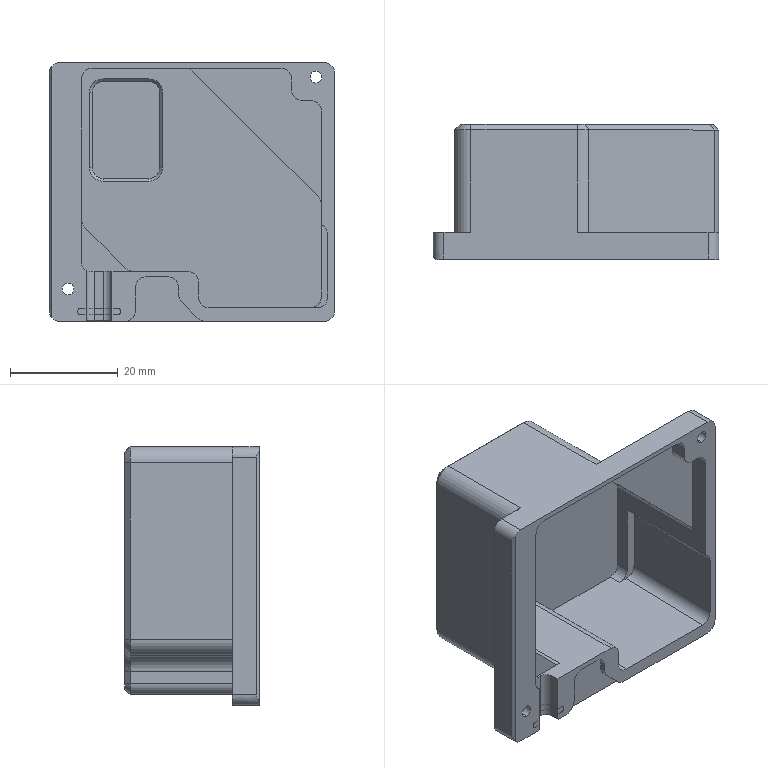NC program | NX | posted with a generic post | part box 53 x 25 x 48 mm
Lines 1678 to 3424 of 6007:
(PLANAR_MILL_3 , TOOL : D4-12-D4-50-3T-ROUGH)
N3348 T09 M6
N3350 G54
N3352 G17 G0 G90 X-17.741 Y0.375 B0. C0. S3000 M3
N3354 G43 Z30. H9
N3356 Z1.004 B-180. C-180.
N3358 G94 G1 Z-0.996 F600.
N3360 X-19.005 Y0.525
N3362 X-19.033 Y0.497
N3364 X-20.9 Y-1.37
N3366 Y-4.009
N3368 Y-4.049
N3370 X-19.9 Y-4.838
N3372 Z1.004
N3374 G0 X-17.741 Y0.375 Z0.009
N3376 G1 Z-1.991
N3378 X-19.005 Y0.525
N3380 X-19.033 Y0.497
N3382 X-20.9 Y-1.37
N3384 Y-4.009
N3386 Y-4.049
N3388 X-19.9 Y-4.838
N3390 Z0.009
N3392 G0 X-17.741 Y0.375 Z-0.987
N3394 G1 Z-2.987
N3396 X-19.005 Y0.525
N3398 X-19.033 Y0.497
N3400 X-20.9 Y-1.37
N3402 Y-4.009
N3404 Y-4.049
N3406 X-19.9 Y-4.838
N3408 Z-0.987
N3410 G0 X-17.741 Y0.375 Z-1.983
N3412 G1 Z-3.983
N3414 X-19.005 Y0.525
N3416 X-19.033 Y0.497
N3418 X-20.9 Y-1.37
N3420 Y-4.009
N3422 Y-4.049
N3424 X-19.9 Y-4.838
N3426 Z-1.983
N3428 G0 X-17.741 Y0.375 Z-2.978
N3430 G1 Z-4.978
N3432 X-19.005 Y0.525
N3434 X-19.033 Y0.497
N3436 X-20.9 Y-1.37
N3438 Y-4.009
N3440 Y-4.049
N3442 X-19.9 Y-4.838
N3444 Z-2.978
N3446 G0 X-17.741 Y0.375 Z-3.974
N3448 G1 Z-5.974
N3450 X-19.005 Y0.525
N3452 X-19.033 Y0.497
N3454 X-20.9 Y-1.37
N3456 Y-4.009
N3458 Y-4.049
N3460 X-19.9 Y-4.838
N3462 Z-3.974
N3464 G0 X-17.741 Y0.375 Z-4.97
N3466 G1 Z-6.97
N3468 X-19.005 Y0.525
N3470 X-19.033 Y0.497
N3472 X-20.9 Y-1.37
N3474 Y-4.009
N3476 Y-4.049
N3478 X-19.9 Y-4.838
N3480 Z-4.97
N3482 G0 X-17.741 Y0.375 Z-5.965
N3484 G1 Z-7.965
N3486 X-19.005 Y0.525
N3488 X-19.033 Y0.497
N3490 X-20.9 Y-1.37
N3492 Y-4.009
N3494 Y-4.049
N3496 X-19.9 Y-4.838
N3498 Z-5.965
N3500 G0 X-17.741 Y0.375 Z-6.961
N3502 G1 Z-8.961
N3504 X-19.005 Y0.525
N3506 X-19.033 Y0.497
N3508 X-20.9 Y-1.37
N3510 Y-4.009
N3512 Y-4.049
N3514 X-19.9 Y-4.838
N3516 Z-6.961
N3518 G0 X-17.741 Y0.375 Z-7.957
N3520 G1 Z-9.957
N3522 X-19.005 Y0.525
N3524 X-19.033 Y0.497
N3526 X-20.9 Y-1.37
N3528 Y-4.009
N3530 Y-4.049
N3532 X-19.9 Y-4.838
N3534 Z-7.957
N3536 G0 X-17.741 Y0.375 Z-8.952
N3538 G1 Z-10.952
N3540 X-19.005 Y0.525
N3542 X-19.033 Y0.497
N3544 X-20.9 Y-1.37
N3546 Y-4.009
N3548 Y-4.049
N3550 X-19.9 Y-4.838
N3552 Z-8.952
N3554 G0 X-17.741 Y0.375 Z-9.948
N3556 G1 Z-11.948
N3558 X-19.005 Y0.525
N3560 X-19.033 Y0.497
N3562 X-20.9 Y-1.37
N3564 Y-4.009
N3566 Y-4.049
N3568 X-19.9 Y-4.838
N3570 Z-9.948
N3572 G0 X-17.741 Y0.375 Z-10.943
N3574 G1 Z-12.943
N3576 X-19.005 Y0.525
N3578 X-19.033 Y0.497
N3580 X-20.9 Y-1.37
N3582 Y-4.009
N3584 Y-4.049
N3586 X-19.9 Y-4.838
N3588 Z-10.943
N3590 G0 X-17.741 Y0.375 Z-11.939
N3592 G1 Z-13.939
N3594 X-19.005 Y0.525
N3596 X-19.033 Y0.497
N3598 X-20.9 Y-1.37
N3600 Y-4.009
N3602 Y-4.049
N3604 X-19.9 Y-4.838
N3606 Z-11.939
N3608 G0 X-17.741 Y0.375 Z-12.935
N3610 G1 Z-14.935
N3612 X-19.005 Y0.525
N3614 X-19.033 Y0.497
N3616 X-20.9 Y-1.37
N3618 Y-4.009
N3620 Y-4.049
N3622 X-19.9 Y-4.838
N3624 Z-12.935
N3626 G0 X-17.741 Y0.375 Z-13.93
N3628 G1 Z-15.93
N3630 X-19.005 Y0.525
N3632 X-19.033 Y0.497
N3634 X-20.9 Y-1.37
N3636 Y-4.009
N3638 Y-4.049
N3640 X-19.9 Y-4.838
N3642 Z-13.93
N3644 G0 X-17.741 Y0.375 Z-14.926
N3646 G1 Z-16.926
N3648 X-19.005 Y0.525
N3650 X-19.033 Y0.497
N3652 X-20.9 Y-1.37
N3654 Y-4.009
N3656 Y-4.049
N3658 X-19.9 Y-4.838
N3660 Z-14.926
N3662 G0 X-17.741 Y0.375 Z-15.922
N3664 G1 Z-17.922
N3666 X-19.005 Y0.525
N3668 X-19.033 Y0.497
N3670 X-20.9 Y-1.37
N3672 Y-4.009
N3674 Y-4.049
N3676 X-19.9 Y-4.838
N3678 Z-15.922
N3680 G0 X-17.741 Y0.375 Z-16.917
N3682 G1 Z-18.917
N3684 X-19.005 Y0.525
N3686 X-19.033 Y0.497
N3688 X-20.9 Y-1.37
N3690 Y-4.009
N3692 Y-4.049
N3694 X-19.9 Y-4.838
N3696 Z-16.917
N3698 G0 X-17.741 Y0.375 Z-17.913
N3700 G1 Z-19.913
N3702 X-19.005 Y0.525
N3704 X-19.033 Y0.497
N3706 X-20.9 Y-1.37
N3708 Y-4.009
N3710 Y-4.049
N3712 X-19.9 Y-4.838
N3714 Z-17.913
N3716 G0 X-17.741 Y0.375 Z-18.909
N3718 G1 Z-20.909
N3720 X-19.005 Y0.525
N3722 X-19.033 Y0.497
N3724 X-20.9 Y-1.37
N3726 Y-4.009
N3728 Y-4.049
N3730 X-19.9 Y-4.838
N3732 Z-18.909
N3734 G0 X-17.741 Y0.375 Z-19.904
N3736 G1 Z-21.904
N3738 X-19.005 Y0.525
N3740 X-19.033 Y0.497
N3742 X-20.9 Y-1.37
N3744 Y-4.009
N3746 Y-4.049
N3748 X-19.9 Y-4.838
N3750 Z-19.904
N3752 G0 X-17.741 Y0.375 Z-20.9
N3754 G1 Z-22.9
N3756 X-19.005 Y0.525
N3758 X-19.033 Y0.497
N3760 X-20.9 Y-1.37
N3762 Y-4.009
N3764 Y-4.049
N3766 X-19.9 Y-4.838
N3768 Z-20.9
N3770 G0 Z3.
N3772 Y-13.175
N3774 Z1.004
N3776 G1 Z-0.996
N3778 X-20.9 Y-13.963
N3780 Y-14.003
N3782 Y-18.4
N3784 X-16.503
N3786 X-16.463
N3788 X-15.675 Y-17.4
N3790 Z1.004
N3792 G0 X-19.9 Y-13.175 Z0.009
N3794 G1 Z-1.991
N3796 X-20.9 Y-13.963
N3798 Y-14.003
N3800 Y-18.4
N3802 X-16.503
N3804 X-16.463
N3806 X-15.675 Y-17.4
N3808 Z0.009
N3810 G0 X-19.9 Y-13.175 Z-0.987
N3812 G1 Z-2.987
N3814 X-20.9 Y-13.963
N3816 Y-14.003
N3818 Y-18.4
N3820 X-16.503
N3822 X-16.463
N3824 X-15.675 Y-17.4
N3826 Z-0.987
N3828 G0 X-19.9 Y-13.175 Z-1.983
N3830 G1 Z-3.983
N3832 X-20.9 Y-13.963
N3834 Y-14.003
N3836 Y-18.4
N3838 X-16.503
N3840 X-16.463
N3842 X-15.675 Y-17.4
N3844 Z-1.983
N3846 G0 X-19.9 Y-13.175 Z-2.978
N3848 G1 Z-4.978
N3850 X-20.9 Y-13.963
N3852 Y-14.003
N3854 Y-18.4
N3856 X-16.503
N3858 X-16.463
N3860 X-15.675 Y-17.4
N3862 Z-2.978
N3864 G0 X-19.9 Y-13.175 Z-3.974
N3866 G1 Z-5.974
N3868 X-20.9 Y-13.963
N3870 Y-14.003
N3872 Y-18.4
N3874 X-16.503
N3876 X-16.463
N3878 X-15.675 Y-17.4
N3880 Z-3.974
N3882 G0 X-19.9 Y-13.175 Z-4.97
N3884 G1 Z-6.97
N3886 X-20.9 Y-13.963
N3888 Y-14.003
N3890 Y-18.4
N3892 X-16.503
N3894 X-16.463
N3896 X-15.675 Y-17.4
N3898 Z-4.97
N3900 G0 X-19.9 Y-13.175 Z-5.965
N3902 G1 Z-7.965
N3904 X-20.9 Y-13.963
N3906 Y-14.003
N3908 Y-18.4
N3910 X-16.503
N3912 X-16.463
N3914 X-15.675 Y-17.4
N3916 Z-5.965
N3918 G0 X-19.9 Y-13.175 Z-6.961
N3920 G1 Z-8.961
N3922 X-20.9 Y-13.963
N3924 Y-14.003
N3926 Y-18.4
N3928 X-16.503
N3930 X-16.463
N3932 X-15.675 Y-17.4
N3934 Z-6.961
N3936 G0 X-19.9 Y-13.175 Z-7.957
N3938 G1 Z-9.957
N3940 X-20.9 Y-13.963
N3942 Y-14.003
N3944 Y-18.4
N3946 X-16.503
N3948 X-16.463
N3950 X-15.675 Y-17.4
N3952 Z-7.957
N3954 G0 X-19.9 Y-13.175 Z-8.952
N3956 G1 Z-10.952
N3958 X-20.9 Y-13.963
N3960 Y-14.003
N3962 Y-18.4
N3964 X-16.503
N3966 X-16.463
N3968 X-15.675 Y-17.4
N3970 Z-8.952
N3972 G0 X-19.9 Y-13.175 Z-9.948
N3974 G1 Z-11.948
N3976 X-20.9 Y-13.963
N3978 Y-14.003
N3980 Y-18.4
N3982 X-16.503
N3984 X-16.463
N3986 X-15.675 Y-17.4
N3988 Z-9.948
N3990 G0 X-19.9 Y-13.175 Z-10.943
N3992 G1 Z-12.943
N3994 X-20.9 Y-13.963
N3996 Y-14.003
N3998 Y-18.4
N4000 X-16.503
N4002 X-16.463
N4004 X-15.675 Y-17.4
N4006 Z-10.943
N4008 G0 X-19.9 Y-13.175 Z-11.939
N4010 G1 Z-13.939
N4012 X-20.9 Y-13.963
N4014 Y-14.003
N4016 Y-18.4
N4018 X-16.503
N4020 X-16.463
N4022 X-15.675 Y-17.4
N4024 Z-11.939
N4026 G0 X-19.9 Y-13.175 Z-12.935
N4028 G1 Z-14.935
N4030 X-20.9 Y-13.963
N4032 Y-14.003
N4034 Y-18.4
N4036 X-16.503
N4038 X-16.463
N4040 X-15.675 Y-17.4
N4042 Z-12.935
N4044 G0 X-19.9 Y-13.175 Z-13.93
N4046 G1 Z-15.93
N4048 X-20.9 Y-13.963
N4050 Y-14.003
N4052 Y-18.4
N4054 X-16.503
N4056 X-16.463
N4058 X-15.675 Y-17.4
N4060 Z-13.93
N4062 G0 X-19.9 Y-13.175 Z-14.926
N4064 G1 Z-16.926
N4066 X-20.9 Y-13.963
N4068 Y-14.003
N4070 Y-18.4
N4072 X-16.503
N4074 X-16.463
N4076 X-15.675 Y-17.4
N4078 Z-14.926
N4080 G0 X-19.9 Y-13.175 Z-15.922
N4082 G1 Z-17.922
N4084 X-20.9 Y-13.963
N4086 Y-14.003
N4088 Y-18.4
N4090 X-16.503
N4092 X-16.463
N4094 X-15.675 Y-17.4
N4096 Z-15.922
N4098 G0 X-19.9 Y-13.175 Z-16.917
N4100 G1 Z-18.917
N4102 X-20.9 Y-13.963
N4104 Y-14.003
N4106 Y-18.4
N4108 X-16.503
N4110 X-16.463
N4112 X-15.675 Y-17.4
N4114 Z-16.917
N4116 G0 X-19.9 Y-13.175 Z-17.913
N4118 G1 Z-19.913
N4120 X-20.9 Y-13.963
N4122 Y-14.003
N4124 Y-18.4
N4126 X-16.503
N4128 X-16.463
N4130 X-15.675 Y-17.4
N4132 Z-17.913
N4134 G0 X-19.9 Y-13.175 Z-18.909
N4136 G1 Z-20.909
N4138 X-20.9 Y-13.963
N4140 Y-14.003
N4142 Y-18.4
N4144 X-16.503
N4146 X-16.463
N4148 X-15.675 Y-17.4
N4150 Z-18.909
N4152 G0 X-19.9 Y-13.175 Z-19.904
N4154 G1 Z-21.904
N4156 X-20.9 Y-13.963
N4158 Y-14.003
N4160 Y-18.4
N4162 X-16.503
N4164 X-16.463
N4166 X-15.675 Y-17.4
N4168 Z-19.904
N4170 G0 X-19.9 Y-13.175 Z-20.9
N4172 G1 Z-22.9
N4174 X-20.9 Y-13.963
N4176 Y-14.003
N4178 Y-18.4
N4180 X-16.503
N4182 X-16.463
N4184 X-15.675 Y-17.4
N4186 Z-20.9
N4188 G0 Z3.
N4190 X1.662
N4192 Z1.004
N4194 G1 Z-0.996
N4196 X2.451 Y-18.4
N4198 X2.491
N4200 X5.13
N4202 X6.997 Y-16.533
N4204 X7.025 Y-16.505
N4206 X6.875 Y-15.241
N4208 Z1.004
N4210 G0 X1.662 Y-17.4 Z0.009
N4212 G1 Z-1.991
N4214 X2.451 Y-18.4
N4216 X2.491
N4218 X5.13
N4220 X6.997 Y-16.533
N4222 X7.025 Y-16.505
N4224 X6.875 Y-15.241
N4226 Z0.009
N4228 G0 X1.662 Y-17.4 Z-0.987
N4230 G1 Z-2.987
N4232 X2.451 Y-18.4
N4234 X2.491
N4236 X5.13
N4238 X6.997 Y-16.533
N4240 X7.025 Y-16.505
N4242 X6.875 Y-15.241
N4244 Z-0.987
N4246 G0 X1.662 Y-17.4 Z-1.983
N4248 G1 Z-3.983
N4250 X2.451 Y-18.4
N4252 X2.491
N4254 X5.13
N4256 X6.997 Y-16.533
N4258 X7.025 Y-16.505
N4260 X6.875 Y-15.241
N4262 Z-1.983
N4264 G0 X1.662 Y-17.4 Z-2.978
N4266 G1 Z-4.978
N4268 X2.451 Y-18.4
N4270 X2.491
N4272 X5.13
N4274 X6.997 Y-16.533
N4276 X7.025 Y-16.505
N4278 X6.875 Y-15.241
N4280 Z-2.978
N4282 G0 X1.662 Y-17.4 Z-3.974
N4284 G1 Z-5.974
N4286 X2.451 Y-18.4
N4288 X2.491
N4290 X5.13
N4292 X6.997 Y-16.533
N4294 X7.025 Y-16.505
N4296 X6.875 Y-15.241
N4298 Z-3.974
N4300 G0 X1.662 Y-17.4 Z-4.97
N4302 G1 Z-6.97
N4304 X2.451 Y-18.4
N4306 X2.491
N4308 X5.13
N4310 X6.997 Y-16.533
N4312 X7.025 Y-16.505
N4314 X6.875 Y-15.241
N4316 Z-4.97
N4318 G0 X1.662 Y-17.4 Z-5.965
N4320 G1 Z-7.965
N4322 X2.451 Y-18.4
N4324 X2.491
N4326 X5.13
N4328 X6.997 Y-16.533
N4330 X7.025 Y-16.505
N4332 X6.875 Y-15.241
N4334 Z-5.965
N4336 G0 X1.662 Y-17.4 Z-6.961
N4338 G1 Z-8.961
N4340 X2.451 Y-18.4
N4342 X2.491
N4344 X5.13
N4346 X6.997 Y-16.533
N4348 X7.025 Y-16.505
N4350 X6.875 Y-15.241
N4352 Z-6.961
N4354 G0 X1.662 Y-17.4 Z-7.957
N4356 G1 Z-9.957
N4358 X2.451 Y-18.4
N4360 X2.491
N4362 X5.13
N4364 X6.997 Y-16.533
N4366 X7.025 Y-16.505
N4368 X6.875 Y-15.241
N4370 Z-7.957
N4372 G0 X1.662 Y-17.4 Z-8.952
N4374 G1 Z-10.952
N4376 X2.451 Y-18.4
N4378 X2.491
N4380 X5.13
N4382 X6.997 Y-16.533
N4384 X7.025 Y-16.505
N4386 X6.875 Y-15.241
N4388 Z-8.952
N4390 G0 X1.662 Y-17.4 Z-9.948
N4392 G1 Z-11.948
N4394 X2.451 Y-18.4
N4396 X2.491
N4398 X5.13
N4400 X6.997 Y-16.533
N4402 X7.025 Y-16.505
N4404 X6.875 Y-15.241
N4406 Z-9.948
N4408 G0 X1.662 Y-17.4 Z-10.943
N4410 G1 Z-12.943
N4412 X2.451 Y-18.4
N4414 X2.491
N4416 X5.13
N4418 X6.997 Y-16.533
N4420 X7.025 Y-16.505
N4422 X6.875 Y-15.241
N4424 Z-10.943
N4426 G0 X1.662 Y-17.4 Z-11.939
N4428 G1 Z-13.939
N4430 X2.451 Y-18.4
N4432 X2.491
N4434 X5.13
N4436 X6.997 Y-16.533
N4438 X7.025 Y-16.505
N4440 X6.875 Y-15.241
N4442 Z-11.939
N4444 G0 X1.662 Y-17.4 Z-12.935
N4446 G1 Z-14.935
N4448 X2.451 Y-18.4
N4450 X2.491
N4452 X5.13
N4454 X6.997 Y-16.533
N4456 X7.025 Y-16.505
N4458 X6.875 Y-15.241
N4460 Z-12.935
N4462 G0 X1.662 Y-17.4 Z-13.93
N4464 G1 Z-15.93
N4466 X2.451 Y-18.4
N4468 X2.491
N4470 X5.13
N4472 X6.997 Y-16.533
N4474 X7.025 Y-16.505
N4476 X6.875 Y-15.241
N4478 Z-13.93
N4480 G0 X1.662 Y-17.4 Z-14.926
N4482 G1 Z-16.926
N4484 X2.451 Y-18.4
N4486 X2.491
N4488 X5.13
N4490 X6.997 Y-16.533
N4492 X7.025 Y-16.505
N4494 X6.875 Y-15.241
N4496 Z-14.926
N4498 G0 X1.662 Y-17.4 Z-15.922
N4500 G1 Z-17.922
N4502 X2.451 Y-18.4
N4504 X2.491
N4506 X5.13
N4508 X6.997 Y-16.533
N4510 X7.025 Y-16.505
N4512 X6.875 Y-15.241
N4514 Z-15.922
N4516 G0 X1.662 Y-17.4 Z-16.917
N4518 G1 Z-18.917
N4520 X2.451 Y-18.4
N4522 X2.491
N4524 X5.13
N4526 X6.997 Y-16.533
N4528 X7.025 Y-16.505
N4530 X6.875 Y-15.241
N4532 Z-16.917
N4534 G0 X1.662 Y-17.4 Z-17.913
N4536 G1 Z-19.913
N4538 X2.451 Y-18.4
N4540 X2.491
N4542 X5.13
N4544 X6.997 Y-16.533
N4546 X7.025 Y-16.505
N4548 X6.875 Y-15.241
N4550 Z-17.913
N4552 G0 X1.662 Y-17.4 Z-18.909
N4554 G1 Z-20.909
N4556 X2.451 Y-18.4
N4558 X2.491
N4560 X5.13
N4562 X6.997 Y-16.533
N4564 X7.025 Y-16.505
N4566 X6.875 Y-15.241
N4568 Z-18.909
N4570 G0 X1.662 Y-17.4 Z-19.904
N4572 G1 Z-21.904
N4574 X2.451 Y-18.4
N4576 X2.491
N4578 X5.13
N4580 X6.997 Y-16.533
N4582 X7.025 Y-16.505
N4584 X6.875 Y-15.241
N4586 Z-19.904
N4588 G0 X1.662 Y-17.4 Z-20.9
N4590 G1 Z-22.9
N4592 X2.451 Y-18.4
N4594 X2.491
N4596 X5.13
N4598 X6.997 Y-16.533
N4600 X7.025 Y-16.505
N4602 X6.875 Y-15.241
N4604 Z-20.9
N4606 G0 Z3.
N4608 X9.491 Y-12.625
N4610 Z1.004
N4612 G1 Z-0.996
N4614 X10.755 Y-12.775
N4616 X10.783 Y-12.747
N4618 X12.65 Y-10.88
N4620 Y-8.241
N4622 Y-8.201
N4624 X11.65 Y-7.412
N4626 Z1.004
N4628 G0 X9.491 Y-12.625 Z0.009
N4630 G1 Z-1.991
N4632 X10.755 Y-12.775
N4634 X10.783 Y-12.747
N4636 X12.65 Y-10.88
N4638 Y-8.241
N4640 Y-8.201
N4642 X11.65 Y-7.412
N4644 Z0.009
N4646 G0 X9.491 Y-12.625 Z-0.987
N4648 G1 Z-2.987
N4650 X10.755 Y-12.775
N4652 X10.783 Y-12.747
N4654 X12.65 Y-10.88
N4656 Y-8.241
N4658 Y-8.201
N4660 X11.65 Y-7.412
N4662 Z-0.987
N4664 G0 X9.491 Y-12.625 Z-1.983
N4666 G1 Z-3.983
N4668 X10.755 Y-12.775
N4670 X10.783 Y-12.747
N4672 X12.65 Y-10.88
N4674 Y-8.241
N4676 Y-8.201
N4678 X11.65 Y-7.412
N4680 Z-1.983
N4682 G0 X9.491 Y-12.625 Z-2.978
N4684 G1 Z-4.978
N4686 X10.755 Y-12.775
N4688 X10.783 Y-12.747
N4690 X12.65 Y-10.88
N4692 Y-8.241
N4694 Y-8.201
N4696 X11.65 Y-7.412
N4698 Z-2.978
N4700 G0 X9.491 Y-12.625 Z-3.974
N4702 G1 Z-5.974
N4704 X10.755 Y-12.775
N4706 X10.783 Y-12.747
N4708 X12.65 Y-10.88
N4710 Y-8.241
N4712 Y-8.201
N4714 X11.65 Y-7.412
N4716 Z-3.974
N4718 G0 X9.491 Y-12.625 Z-4.97
N4720 G1 Z-6.97
N4722 X10.755 Y-12.775
N4724 X10.783 Y-12.747
N4726 X12.65 Y-10.88
N4728 Y-8.241
N4730 Y-8.201
N4732 X11.65 Y-7.412
N4734 Z-4.97
N4736 G0 X9.491 Y-12.625 Z-5.965
N4738 G1 Z-7.965
N4740 X10.755 Y-12.775
N4742 X10.783 Y-12.747
N4744 X12.65 Y-10.88
N4746 Y-8.241
N4748 Y-8.201
N4750 X11.65 Y-7.412
N4752 Z-5.965
N4754 G0 X9.491 Y-12.625 Z-6.961
N4756 G1 Z-8.961
N4758 X10.755 Y-12.775
N4760 X10.783 Y-12.747
N4762 X12.65 Y-10.88
N4764 Y-8.241
N4766 Y-8.201
N4768 X11.65 Y-7.412
N4770 Z-6.961
N4772 G0 X9.491 Y-12.625 Z-7.957
N4774 G1 Z-9.957
N4776 X10.755 Y-12.775
N4778 X10.783 Y-12.747
N4780 X12.65 Y-10.88
N4782 Y-8.241
N4784 Y-8.201
N4786 X11.65 Y-7.412
N4788 Z-7.957
N4790 G0 X9.491 Y-12.625 Z-8.952
N4792 G1 Z-10.952
N4794 X10.755 Y-12.775
N4796 X10.783 Y-12.747
N4798 X12.65 Y-10.88
N4800 Y-8.241
N4802 Y-8.201
N4804 X11.65 Y-7.412
N4806 Z-8.952
N4808 G0 X9.491 Y-12.625 Z-9.948
N4810 G1 Z-11.948
N4812 X10.755 Y-12.775
N4814 X10.783 Y-12.747
N4816 X12.65 Y-10.88
N4818 Y-8.241
N4820 Y-8.201
N4822 X11.65 Y-7.412
N4824 Z-9.948
N4826 G0 X9.491 Y-12.625 Z-10.943
N4828 G1 Z-12.943
N4830 X10.755 Y-12.775
N4832 X10.783 Y-12.747
N4834 X12.65 Y-10.88
N4836 Y-8.241
N4838 Y-8.201
N4840 X11.65 Y-7.412
N4842 Z-10.943
N4844 G0 X9.491 Y-12.625 Z-11.939
N4846 G1 Z-13.939
N4848 X10.755 Y-12.775
N4850 X10.783 Y-12.747
N4852 X12.65 Y-10.88
N4854 Y-8.241
N4856 Y-8.201
N4858 X11.65 Y-7.412
N4860 Z-11.939
N4862 G0 X9.491 Y-12.625 Z-12.935
N4864 G1 Z-14.935
N4866 X10.755 Y-12.775
N4868 X10.783 Y-12.747
N4870 X12.65 Y-10.88
N4872 Y-8.241
N4874 Y-8.201
N4876 X11.65 Y-7.412
N4878 Z-12.935
N4880 G0 X9.491 Y-12.625 Z-13.93
N4882 G1 Z-15.93
N4884 X10.755 Y-12.775
N4886 X10.783 Y-12.747
N4888 X12.65 Y-10.88
N4890 Y-8.241
N4892 Y-8.201
N4894 X11.65 Y-7.412
N4896 Z-13.93
N4898 G0 X9.491 Y-12.625 Z-14.926
N4900 G1 Z-16.926
N4902 X10.755 Y-12.775
N4904 X10.783 Y-12.747
N4906 X12.65 Y-10.88
N4908 Y-8.241
N4910 Y-8.201
N4912 X11.65 Y-7.412
N4914 Z-14.926
N4916 G0 X9.491 Y-12.625 Z-15.922
N4918 G1 Z-17.922
N4920 X10.755 Y-12.775
N4922 X10.783 Y-12.747
N4924 X12.65 Y-10.88
N4926 Y-8.241
N4928 Y-8.201
N4930 X11.65 Y-7.412
N4932 Z-15.922
N4934 G0 X9.491 Y-12.625 Z-16.917
N4936 G1 Z-18.917
N4938 X10.755 Y-12.775
N4940 X10.783 Y-12.747
N4942 X12.65 Y-10.88
N4944 Y-8.241
N4946 Y-8.201
N4948 X11.65 Y-7.412
N4950 Z-16.917
N4952 G0 X9.491 Y-12.625 Z-17.913
N4954 G1 Z-19.913
N4956 X10.755 Y-12.775
N4958 X10.783 Y-12.747
N4960 X12.65 Y-10.88
N4962 Y-8.241
N4964 Y-8.201
N4966 X11.65 Y-7.412
N4968 Z-17.913
N4970 G0 X9.491 Y-12.625 Z-18.909
N4972 G1 Z-20.909
N4974 X10.755 Y-12.775
N4976 X10.783 Y-12.747
N4978 X12.65 Y-10.88
N4980 Y-8.241
N4982 Y-8.201
N4984 X11.65 Y-7.412
N4986 Z-18.909
N4988 G0 X9.491 Y-12.625 Z-19.904
N4990 G1 Z-21.904
N4992 X10.755 Y-12.775
N4994 X10.783 Y-12.747
N4996 X12.65 Y-10.88
N4998 Y-8.241
N5000 Y-8.201
N5002 X11.65 Y-7.412
N5004 Z-19.904
N5006 G0 X9.491 Y-12.625 Z-20.9
N5008 G1 Z-22.9
N5010 X10.755 Y-12.775
N5012 X10.783 Y-12.747
N5014 X12.65 Y-10.88
N5016 Y-8.241
N5018 Y-8.201
N5020 X11.65 Y-7.412
N5022 Z-20.9
N5024 G0 Z3.
N5026 X14.053 Y3.529
N5028 Z1.004
N5030 G1 Z-0.996
N5032 X15.04 Y2.927
N5034 X15.077 Y2.943
N5036 G2 X16.75 Y3.3 R4.1
N5038 G1 X19.4
N5040 Y7.688
N5042 Y7.728
N5044 X18.4 Y8.517
N5046 Z1.004
N5048 G0 X14.053 Y3.529 Z0.009
N5050 G1 Z-1.991
N5052 X15.04 Y2.927
N5054 X15.077 Y2.943
N5056 G2 X16.75 Y3.3 R4.1
N5058 G1 X19.4
N5060 Y7.688
N5062 Y7.728
N5064 X18.4 Y8.517
N5066 Z0.009
N5068 G0 X14.053 Y3.529 Z-0.987
N5070 G1 Z-2.987
N5072 X15.04 Y2.927
N5074 X15.077 Y2.943
N5076 G2 X16.75 Y3.3 R4.1
N5078 G1 X19.4
N5080 Y7.688
N5082 Y7.728
N5084 X18.4 Y8.517
N5086 Z-0.987
N5088 G0 X14.053 Y3.529 Z-1.983
N5090 G1 Z-3.983
N5092 X15.04 Y2.927
N5094 X15.077 Y2.943
N5096 G2 X16.75 Y3.3 R4.1
N5098 G1 X19.4
N5100 Y7.688
N5102 Y7.728
N5104 X18.4 Y8.517
N5106 Z-1.983
N5108 G0 X14.053 Y3.529 Z-2.978
N5110 G1 Z-4.978
N5112 X15.04 Y2.927
N5114 X15.077 Y2.943
N5116 G2 X16.75 Y3.3 R4.1
N5118 G1 X19.4
N5120 Y7.688
N5122 Y7.728
N5124 X18.4 Y8.517
N5126 Z-2.978
N5128 G0 X14.053 Y3.529 Z-3.974
N5130 G1 Z-5.974
N5132 X15.04 Y2.927
N5134 X15.077 Y2.943
N5136 G2 X16.75 Y3.3 R4.1
N5138 G1 X19.4
N5140 Y7.688
N5142 Y7.728
N5144 X18.4 Y8.517
N5146 Z-3.974
N5148 G0 X14.053 Y3.529 Z-4.97
N5150 G1 Z-6.97
N5152 X15.04 Y2.927
N5154 X15.077 Y2.943
N5156 G2 X16.75 Y3.3 R4.1
N5158 G1 X19.4
N5160 Y7.688
N5162 Y7.728
N5164 X18.4 Y8.517
N5166 Z-4.97
N5168 G0 X14.053 Y3.529 Z-5.965
N5170 G1 Z-7.965
N5172 X15.04 Y2.927
N5174 X15.077 Y2.943
N5176 G2 X16.75 Y3.3 R4.1
N5178 G1 X19.4
N5180 Y7.688
N5182 Y7.728
N5184 X18.4 Y8.517
N5186 Z-5.965
N5188 G0 X14.053 Y3.529 Z-6.961
N5190 G1 Z-8.961
N5192 X15.04 Y2.927
N5194 X15.077 Y2.943
N5196 G2 X16.75 Y3.3 R4.1
N5198 G1 X19.4
N5200 Y7.688
N5202 Y7.728
N5204 X18.4 Y8.517
N5206 Z-6.961
N5208 G0 X14.053 Y3.529 Z-7.957
N5210 G1 Z-9.957
N5212 X15.04 Y2.927
N5214 X15.077 Y2.943
N5216 G2 X16.75 Y3.3 R4.1
N5218 G1 X19.4
N5220 Y7.688
N5222 Y7.728
N5224 X18.4 Y8.517
N5226 Z-7.957
N5228 G0 X14.053 Y3.529 Z-8.952
N5230 G1 Z-10.952
N5232 X15.04 Y2.927
N5234 X15.077 Y2.943
N5236 G2 X16.75 Y3.3 R4.1
N5238 G1 X19.4
N5240 Y7.688
N5242 Y7.728
N5244 X18.4 Y8.517
N5246 Z-8.952
N5248 G0 X14.053 Y3.529 Z-9.948
N5250 G1 Z-11.948
N5252 X15.04 Y2.927
N5254 X15.077 Y2.943
N5256 G2 X16.75 Y3.3 R4.1
N5258 G1 X19.4
N5260 Y7.688
N5262 Y7.728
N5264 X18.4 Y8.517
N5266 Z-9.948
N5268 G0 X14.053 Y3.529 Z-10.943
N5270 G1 Z-12.943
N5272 X15.04 Y2.927
N5274 X15.077 Y2.943
N5276 G2 X16.75 Y3.3 R4.1
N5278 G1 X19.4
N5280 Y7.688
N5282 Y7.728
N5284 X18.4 Y8.517
N5286 Z-10.943
N5288 G0 X14.053 Y3.529 Z-11.939
N5290 G1 Z-13.939
N5292 X15.04 Y2.927
N5294 X15.077 Y2.943
N5296 G2 X16.75 Y3.3 R4.1
N5298 G1 X19.4
N5300 Y7.688
N5302 Y7.728
N5304 X18.4 Y8.517
N5306 Z-11.939
N5308 G0 X14.053 Y3.529 Z-12.935
N5310 G1 Z-14.935
N5312 X15.04 Y2.927
N5314 X15.077 Y2.943
N5316 G2 X16.75 Y3.3 R4.1
N5318 G1 X19.4
N5320 Y7.688
N5322 Y7.728
N5324 X18.4 Y8.517
N5326 Z-12.935
N5328 G0 X14.053 Y3.529 Z-13.93
N5330 G1 Z-15.93
N5332 X15.04 Y2.927
N5334 X15.077 Y2.943
N5336 G2 X16.75 Y3.3 R4.1
N5338 G1 X19.4
N5340 Y7.688
N5342 Y7.728
N5344 X18.4 Y8.517
N5346 Z-13.93
N5348 G0 X14.053 Y3.529 Z-14.926
N5350 G1 Z-16.926
N5352 X15.04 Y2.927
N5354 X15.077 Y2.943
N5356 G2 X16.75 Y3.3 R4.1
N5358 G1 X19.4
N5360 Y7.688
N5362 Y7.728
N5364 X18.4 Y8.517
N5366 Z-14.926
N5368 G0 X14.053 Y3.529 Z-15.922
N5370 G1 Z-17.922
N5372 X15.04 Y2.927
N5374 X15.077 Y2.943
N5376 G2 X16.75 Y3.3 R4.1
N5378 G1 X19.4
N5380 Y7.688
N5382 Y7.728
N5384 X18.4 Y8.517
N5386 Z-15.922
N5388 G0 X14.053 Y3.529 Z-16.917
N5390 G1 Z-18.917
N5392 X15.04 Y2.927
N5394 X15.077 Y2.943
N5396 G2 X16.75 Y3.3 R4.1
N5398 G1 X19.4
N5400 Y7.688
N5402 Y7.728
N5404 X18.4 Y8.517
N5406 Z-16.917
N5408 G0 X14.053 Y3.529 Z-17.913
N5410 G1 Z-19.913
N5412 X15.04 Y2.927
N5414 X15.077 Y2.943
N5416 G2 X16.75 Y3.3 R4.1
N5418 G1 X19.4
N5420 Y7.688
N5422 Y7.728
N5424 X18.4 Y8.517
N5426 Z-17.913
N5428 G0 X14.053 Y3.529 Z-18.909
N5430 G1 Z-20.909
N5432 X15.04 Y2.927
N5434 X15.077 Y2.943
N5436 G2 X16.75 Y3.3 R4.1
N5438 G1 X19.4
N5440 Y7.688
N5442 Y7.728
N5444 X18.4 Y8.517
N5446 Z-18.909
N5448 G0 X14.053 Y3.529 Z-19.904
N5450 G1 Z-21.904
N5452 X15.04 Y2.927
N5454 X15.077 Y2.943
N5456 G2 X16.75 Y3.3 R4.1
N5458 G1 X19.4
N5460 Y7.688
N5462 Y7.728
N5464 X18.4 Y8.517
N5466 Z-19.904
N5468 G0 X14.053 Y3.529 Z-20.9
N5470 G1 Z-22.9
N5472 X15.04 Y2.927
N5474 X15.077 Y2.943
N5476 G2 X16.75 Y3.3 R4.1
N5478 G1 X19.4
N5480 Y7.688
N5482 Y7.728
N5484 X18.4 Y8.517
N5486 Z-20.9
N5488 G0 Z3.
N5490 Y16.675
N5492 Z1.004
N5494 G1 Z-0.996
N5496 X19.4 Y17.463
N5498 Y17.503
N5500 Y21.9
N5502 X15.003
N5504 X14.963
N5506 X14.175 Y20.9
N5508 Z1.004
N5510 G0 X18.4 Y16.675 Z0.009
N5512 G1 Z-1.991
N5514 X19.4 Y17.463
N5516 Y17.503
N5518 Y21.9
N5520 X15.003
N5522 X14.963
N5524 X14.175 Y20.9
N5526 Z0.009
N5528 G0 X18.4 Y16.675 Z-0.987
N5530 G1 Z-2.987
N5532 X19.4 Y17.463
N5534 Y17.503
N5536 Y21.9
N5538 X15.003
N5540 X14.963
N5542 X14.175 Y20.9
N5544 Z-0.987
N5546 G0 X18.4 Y16.675 Z-1.983
N5548 G1 Z-3.983
N5550 X19.4 Y17.463
N5552 Y17.503
N5554 Y21.9
N5556 X15.003
N5558 X14.963
N5560 X14.175 Y20.9
N5562 Z-1.983
N5564 G0 X18.4 Y16.675 Z-2.978
N5566 G1 Z-4.978
N5568 X19.4 Y17.463
N5570 Y17.503
N5572 Y21.9
N5574 X15.003
N5576 X14.963
N5578 X14.175 Y20.9
N5580 Z-2.978
N5582 G0 X18.4 Y16.675 Z-3.974
N5584 G1 Z-5.974
N5586 X19.4 Y17.463
N5588 Y17.503
N5590 Y21.9
N5592 X15.003
N5594 X14.963
N5596 X14.175 Y20.9
N5598 Z-3.974
N5600 G0 X18.4 Y16.675 Z-4.97
N5602 G1 Z-6.97
N5604 X19.4 Y17.463
N5606 Y17.503
N5608 Y21.9
N5610 X15.003
N5612 X14.963
N5614 X14.175 Y20.9
N5616 Z-4.97
N5618 G0 X18.4 Y16.675 Z-5.965
N5620 G1 Z-7.965
N5622 X19.4 Y17.463
N5624 Y17.503
N5626 Y21.9
N5628 X15.003
N5630 X14.963
N5632 X14.175 Y20.9
N5634 Z-5.965
N5636 G0 X18.4 Y16.675 Z-6.961
N5638 G1 Z-8.961
N5640 X19.4 Y17.463
N5642 Y17.503
N5644 Y21.9
N5646 X15.003
N5648 X14.963
N5650 X14.175 Y20.9
N5652 Z-6.961
N5654 G0 X18.4 Y16.675 Z-7.957
N5656 G1 Z-9.957
N5658 X19.4 Y17.463
N5660 Y17.503
N5662 Y21.9
N5664 X15.003
N5666 X14.963
N5668 X14.175 Y20.9
N5670 Z-7.957
N5672 G0 X18.4 Y16.675 Z-8.952
N5674 G1 Z-10.952
N5676 X19.4 Y17.463
N5678 Y17.503
N5680 Y21.9
N5682 X15.003
N5684 X14.963
N5686 X14.175 Y20.9
N5688 Z-8.952
N5690 G0 X18.4 Y16.675 Z-9.948
N5692 G1 Z-11.948
N5694 X19.4 Y17.463
N5696 Y17.503
N5698 Y21.9
N5700 X15.003
N5702 X14.963
N5704 X14.175 Y20.9
N5706 Z-9.948
N5708 G0 X18.4 Y16.675 Z-10.943
N5710 G1 Z-12.943
N5712 X19.4 Y17.463
N5714 Y17.503
N5716 Y21.9
N5718 X15.003
N5720 X14.963
N5722 X14.175 Y20.9
N5724 Z-10.943
N5726 G0 X18.4 Y16.675 Z-11.939
N5728 G1 Z-13.939
N5730 X19.4 Y17.463
N5732 Y17.503
N5734 Y21.9
N5736 X15.003
N5738 X14.963
N5740 X14.175 Y20.9
N5742 Z-11.939
N5744 G0 X18.4 Y16.675 Z-12.935
N5746 G1 Z-14.935
N5748 X19.4 Y17.463
N5750 Y17.503
N5752 Y21.9
N5754 X15.003
N5756 X14.963
N5758 X14.175 Y20.9
N5760 Z-12.935
N5762 G0 X18.4 Y16.675 Z-13.93
N5764 G1 Z-15.93
N5766 X19.4 Y17.463
N5768 Y17.503
N5770 Y21.9
N5772 X15.003
N5774 X14.963
N5776 X14.175 Y20.9
N5778 Z-13.93
N5780 G0 X18.4 Y16.675 Z-14.926
N5782 G1 Z-16.926
N5784 X19.4 Y17.463
N5786 Y17.503
N5788 Y21.9
N5790 X15.003
N5792 X14.963
N5794 X14.175 Y20.9
N5796 Z-14.926
N5798 G0 X18.4 Y16.675 Z-15.922
N5800 G1 Z-17.922
N5802 X19.4 Y17.463
N5804 Y17.503
N5806 Y21.9
N5808 X15.003
N5810 X14.963
N5812 X14.175 Y20.9
N5814 Z-15.922
N5816 G0 X18.4 Y16.675 Z-16.917
N5818 G1 Z-18.917
N5820 X19.4 Y17.463
N5822 Y17.503
N5824 Y21.9
N5826 X15.003
N5828 X14.963
N5830 X14.175 Y20.9
N5832 Z-16.917
N5834 G0 X18.4 Y16.675 Z-17.913
N5836 G1 Z-19.913
N5838 X19.4 Y17.463
N5840 Y17.503
N5842 Y21.9
N5844 X15.003
N5846 X14.963
N5848 X14.175 Y20.9
N5850 Z-17.913
N5852 G0 X18.4 Y16.675 Z-18.909
N5854 G1 Z-20.909
N5856 X19.4 Y17.463
N5858 Y17.503
N5860 Y21.9
N5862 X15.003
N5864 X14.963
N5866 X14.175 Y20.9
N5868 Z-18.909
N5870 G0 X18.4 Y16.675 Z-19.904
N5872 G1 Z-21.904
N5874 X19.4 Y17.463
N5876 Y17.503
N5878 Y21.9
N5880 X15.003
N5882 X14.963
N5884 X14.175 Y20.9
N5886 Z-19.904
N5888 G0 X18.4 Y16.675 Z-20.9
N5890 G1 Z-22.9
N5892 X19.4 Y17.463
N5894 Y17.503
N5896 Y21.9
N5898 X15.003
N5900 X14.963
N5902 X14.175 Y20.9
N5904 Z-20.9
N5906 G0 Z3.
N5908 X5.838
N5910 Z1.004
N5912 G1 Z-0.996
N5914 X5.049 Y21.9
N5916 X5.009
N5918 X2.37
N5920 X0.503 Y20.033
N5922 X0.475 Y20.005
N5924 X0.625 Y18.741
N5926 Z1.004
N5928 G0 X5.838 Y20.9 Z0.009
N5930 G1 Z-1.991
N5932 X5.049 Y21.9
N5934 X5.009
N5936 X2.37
N5938 X0.503 Y20.033
N5940 X0.475 Y20.005
N5942 X0.625 Y18.741
N5944 Z0.009
N5946 G0 X5.838 Y20.9 Z-0.987
N5948 G1 Z-2.987
N5950 X5.049 Y21.9
N5952 X5.009
N5954 X2.37
N5956 X0.503 Y20.033
N5958 X0.475 Y20.005
N5960 X0.625 Y18.741
N5962 Z-0.987
N5964 G0 X5.838 Y20.9 Z-1.983
N5966 G1 Z-3.983
N5968 X5.049 Y21.9
N5970 X5.009
N5972 X2.37
N5974 X0.503 Y20.033
N5976 X0.475 Y20.005
N5978 X0.625 Y18.741
N5980 Z-1.983
N5982 G0 X5.838 Y20.9 Z-2.978
N5984 G1 Z-4.978
N5986 X5.049 Y21.9
N5988 X5.009
N5990 X2.37
N5992 X0.503 Y20.033
N5994 X0.475 Y20.005
N5996 X0.625 Y18.741
N5998 Z-2.978
N6000 G0 X5.838 Y20.9 Z-3.974
N6002 G1 Z-5.974
N6004 X5.049 Y21.9
N6006 X5.009
N6008 X2.37
N6010 X0.503 Y20.033
N6012 X0.475 Y20.005
N6014 X0.625 Y18.741
N6016 Z-3.974
N6018 G0 X5.838 Y20.9 Z-4.97
N6020 G1 Z-6.97
N6022 X5.049 Y21.9
N6024 X5.009
N6026 X2.37
N6028 X0.503 Y20.033
N6030 X0.475 Y20.005
N6032 X0.625 Y18.741
N6034 Z-4.97
N6036 G0 X5.838 Y20.9 Z-5.965
N6038 G1 Z-7.965
N6040 X5.049 Y21.9
N6042 X5.009
N6044 X2.37
N6046 X0.503 Y20.033
N6048 X0.475 Y20.005
N6050 X0.625 Y18.741
N6052 Z-5.965
N6054 G0 X5.838 Y20.9 Z-6.961
N6056 G1 Z-8.961
N6058 X5.049 Y21.9
N6060 X5.009
N6062 X2.37
N6064 X0.503 Y20.033
N6066 X0.475 Y20.005
N6068 X0.625 Y18.741
N6070 Z-6.961
N6072 G0 X5.838 Y20.9 Z-7.957
N6074 G1 Z-9.957
N6076 X5.049 Y21.9
N6078 X5.009
N6080 X2.37
N6082 X0.503 Y20.033
N6084 X0.475 Y20.005
N6086 X0.625 Y18.741
N6088 Z-7.957
N6090 G0 X5.838 Y20.9 Z-8.952
N6092 G1 Z-10.952
N6094 X5.049 Y21.9
N6096 X5.009
N6098 X2.37
N6100 X0.503 Y20.033
N6102 X0.475 Y20.005
N6104 X0.625 Y18.741
N6106 Z-8.952
N6108 G0 X5.838 Y20.9 Z-9.948
N6110 G1 Z-11.948
N6112 X5.049 Y21.9
N6114 X5.009
N6116 X2.37
N6118 X0.503 Y20.033
N6120 X0.475 Y20.005
N6122 X0.625 Y18.741
N6124 Z-9.948
N6126 G0 X5.838 Y20.9 Z-10.943
N6128 G1 Z-12.943
N6130 X5.049 Y21.9
N6132 X5.009
N6134 X2.37
N6136 X0.503 Y20.033
N6138 X0.475 Y20.005
N6140 X0.625 Y18.741
N6142 Z-10.943
N6144 G0 X5.838 Y20.9 Z-11.939
N6146 G1 Z-13.939
N6148 X5.049 Y21.9
N6150 X5.009
N6152 X2.37
N6154 X0.503 Y20.033
N6156 X0.475 Y20.005
N6158 X0.625 Y18.741
N6160 Z-11.939
N6162 G0 X5.838 Y20.9 Z-12.935
N6164 G1 Z-14.935
N6166 X5.049 Y21.9
N6168 X5.009
N6170 X2.37
N6172 X0.503 Y20.033
N6174 X0.475 Y20.005
N6176 X0.625 Y18.741
N6178 Z-12.935
N6180 G0 X5.838 Y20.9 Z-13.93
N6182 G1 Z-15.93
N6184 X5.049 Y21.9
N6186 X5.009
N6188 X2.37
N6190 X0.503 Y20.033
N6192 X0.475 Y20.005
N6194 X0.625 Y18.741
N6196 Z-13.93
N6198 G0 X5.838 Y20.9 Z-14.926
N6200 G1 Z-16.926
N6202 X5.049 Y21.9
N6204 X5.009
N6206 X2.37
N6208 X0.503 Y20.033
N6210 X0.475 Y20.005
N6212 X0.625 Y18.741
N6214 Z-14.926
N6216 G0 X5.838 Y20.9 Z-15.922
N6218 G1 Z-17.922
N6220 X5.049 Y21.9
N6222 X5.009
N6224 X2.37
N6226 X0.503 Y20.033
N6228 X0.475 Y20.005
N6230 X0.625 Y18.741
N6232 Z-15.922
N6234 G0 X5.838 Y20.9 Z-16.917
N6236 G1 Z-18.917
N6238 X5.049 Y21.9
N6240 X5.009
N6242 X2.37
N6244 X0.503 Y20.033
N6246 X0.475 Y20.005
N6248 X0.625 Y18.741
N6250 Z-16.917
N6252 G0 X5.838 Y20.9 Z-17.913
N6254 G1 Z-19.913
N6256 X5.049 Y21.9
N6258 X5.009
N6260 X2.37
N6262 X0.503 Y20.033
N6264 X0.475 Y20.005
N6266 X0.625 Y18.741
N6268 Z-17.913
N6270 G0 X5.838 Y20.9 Z-18.909
N6272 G1 Z-20.909
N6274 X5.049 Y21.9
N6276 X5.009
N6278 X2.37
N6280 X0.503 Y20.033
N6282 X0.475 Y20.005
N6284 X0.625 Y18.741
N6286 Z-18.909
N6288 G0 X5.838 Y20.9 Z-19.904
N6290 G1 Z-21.904
N6292 X5.049 Y21.9
N6294 X5.009
N6296 X2.37
N6298 X0.503 Y20.033
N6300 X0.475 Y20.005
N6302 X0.625 Y18.741
N6304 Z-19.904
N6306 G0 X5.838 Y20.9 Z-20.9
N6308 G1 Z-22.9
N6310 X5.049 Y21.9
N6312 X5.009
N6314 X2.37
N6316 X0.503 Y20.033
N6318 X0.475 Y20.005
N6320 X0.625 Y18.741
N6322 Z-20.9
N6324 G0 Z30.
(PLANAR_MILL_3_COPY_COPY , TOOL : D4-12-D4-50-3T-ROUGH)
N6326 X5.253 Y-16.4
N6328 Z1.543
N6330 G1 Z-0.457
N6332 G3 X7.253 Y-18.4 R2.
N6334 G1 X12.65
N6336 Y-13.003
N6338 G3 X10.65 Y-11.003 R2.
N6340 G1 Z1.543
N6342 G0 X5.253 Y-16.4 Z1.086
N6344 G1 Z-0.914
N6346 G3 X7.253 Y-18.4 R2.
N6348 G1 X12.65
N6350 Y-13.003
N6352 G3 X10.65 Y-11.003 R2.
N6354 G1 Z1.086
N6356 G0 X5.253 Y-16.4 Z0.629
N6358 G1 Z-1.371
N6360 G3 X7.253 Y-18.4 R2.
N6362 G1 X12.65
N6364 Y-13.003
N6366 G3 X10.65 Y-11.003 R2.
N6368 G1 Z0.629
N6370 G0 X5.253 Y-16.4 Z0.171
N6372 G1 Z-1.829
N6374 G3 X7.253 Y-18.4 R2.
N6376 G1 X12.65
N6378 Y-13.003
N6380 G3 X10.65 Y-11.003 R2.
N6382 G1 Z0.171
N6384 G0 X5.253 Y-16.4 Z-0.286
N6386 G1 Z-2.286
N6388 G3 X7.253 Y-18.4 R2.
N6390 G1 X12.65
N6392 Y-13.003
N6394 G3 X10.65 Y-11.003 R2.
N6396 G1 Z-0.286
N6398 G0 X5.253 Y-16.4 Z-0.743
N6400 G1 Z-2.743
N6402 G3 X7.253 Y-18.4 R2.
N6404 G1 X12.65
N6406 Y-13.003
N6408 G3 X10.65 Y-11.003 R2.
N6410 G1 Z-0.743
N6412 G0 X5.253 Y-16.4 Z-1.2
N6414 G1 Z-3.2
N6416 G3 X7.253 Y-18.4 R2.
N6418 G1 X12.65
N6420 Y-13.003
N6422 G3 X10.65 Y-11.003 R2.
N6424 G1 Z-1.2
N6426 G0 Z3.
N6428 X-7.686 Y19.9
N6430 Z1.543
N6432 G1 Z-0.457
N6434 G3 X-9.686 Y21.9 R2.
N6436 G1 X-14.9
N6438 Y20.5
N6440 G2 X-19. Y16.4 R4.1
N6442 G1 X-20.9
N6444 Y11.089
N6446 G3 X-18.9 Y9.089 R2.
N6448 G1 Z1.543
N6450 G0 X-7.686 Y19.9 Z1.086
N6452 G1 Z-0.914
N6454 G3 X-9.686 Y21.9 R2.
N6456 G1 X-14.9
N6458 Y20.5
N6460 G2 X-19. Y16.4 R4.1
N6462 G1 X-20.9
N6464 Y11.089
N6466 G3 X-18.9 Y9.089 R2.
N6468 G1 Z1.086
N6470 G0 X-7.686 Y19.9 Z0.629
N6472 G1 Z-1.371
N6474 G3 X-9.686 Y21.9 R2.
N6476 G1 X-14.9
N6478 Y20.5
N6480 G2 X-19. Y16.4 R4.1
N6482 G1 X-20.9
N6484 Y11.089
N6486 G3 X-18.9 Y9.089 R2.
N6488 G1 Z0.629
N6490 G0 X-7.686 Y19.9 Z0.171
N6492 G1 Z-1.829
N6494 G3 X-9.686 Y21.9 R2.
N6496 G1 X-14.9
N6498 Y20.5
N6500 G2 X-19. Y16.4 R4.1
N6502 G1 X-20.9
N6504 Y11.089
N6506 G3 X-18.9 Y9.089 R2.
N6508 G1 Z0.171
N6510 G0 X-7.686 Y19.9 Z-0.286
N6512 G1 Z-2.286
N6514 G3 X-9.686 Y21.9 R2.
N6516 G1 X-14.9
N6518 Y20.5
N6520 G2 X-19. Y16.4 R4.1
N6522 G1 X-20.9
N6524 Y11.089
N6526 G3 X-18.9 Y9.089 R2.
N6528 G1 Z-0.286
N6530 G0 X-7.686 Y19.9 Z-0.743
N6532 G1 Z-2.743
N6534 G3 X-9.686 Y21.9 R2.
N6536 G1 X-14.9
N6538 Y20.5
N6540 G2 X-19. Y16.4 R4.1
N6542 G1 X-20.9
N6544 Y11.089
N6546 G3 X-18.9 Y9.089 R2.
N6548 G1 Z-0.743
N6550 G0 X-7.686 Y19.9 Z-1.2
N6552 G1 Z-3.2
N6554 G3 X-9.686 Y21.9 R2.
N6556 G1 X-14.9
N6558 Y20.5
N6560 G2 X-19. Y16.4 R4.1
N6562 G1 X-20.9
N6564 Y11.089
N6566 G3 X-18.9 Y9.089 R2.
N6568 G1 Z-1.2
N6570 G0 Z30.
(PLANAR_MILL_3_COPY_COPY_COPY , TOOL : D4-12-D4-50-3T-ROUGH)
N6572 X26. Y-5.934
N6574 Z1.55
N6576 G1 Z-0.45
N6578 X24.
N6580 Y-8.921
N6582 G3 X22. Y-8.4 R4.1
N6584 G1 X17.85
N6586 Y-4.6
N6588 X18.972
N6590 G3 X21.871 Y-3.399 R4.1
N6592 G1 X24. Y-1.27
N6594 Y-5.934
N6596 X22.4
N6598 Y-6.814
N6600 G3 X22. Y-6.8 R5.7
N6602 G1 X19.45
N6604 Y-6.18
N6606 G3 X22.4 Y-5.054 R5.7
N6608 G1 Y-5.934
N6610 X24.4
N6612 Z1.55
N6614 G0 X26. Z1.1
N6616 G1 Z-0.9
N6618 X24.
N6620 Y-8.921
N6622 G3 X22. Y-8.4 R4.1
N6624 G1 X17.85
N6626 Y-4.6
N6628 X18.972
N6630 G3 X21.871 Y-3.399 R4.1
N6632 G1 X24. Y-1.27
N6634 Y-5.934
N6636 X22.4
N6638 Y-6.814
N6640 G3 X22. Y-6.8 R5.7
N6642 G1 X19.45
N6644 Y-6.18
N6646 G3 X22.4 Y-5.054 R5.7
N6648 G1 Y-5.934
N6650 X24.4
N6652 Z1.1
N6654 G0 Z30.
(PLANAR_MILL_3_COPY , TOOL : D4-12-D4-50-3T-ROUGH)
N6656 X-11.414 Y-11.3 S4500
N6658 Z-21.5
N6660 G1 X-15.2 Z-21.698
N6662 Y-13.2 Z-21.798
N6664 X-7.8 Z-22.186
N6666 Y-11.3 Z-22.285
N6668 X-15.2 Z-22.673
N6670 Y-13.2 Z-22.773
N6672 X-11.5 Z-22.967
N6674 X-7.8
N6676 Y-11.3
N6678 X-15.2
N6680 Y-13.2
N6682 X-11.5
N6684 Y-14.8
N6686 X-6.2
N6688 Y-9.7
N6690 X-16.8
N6692 Y-14.8
N6694 X-11.5
N6696 Y-16.4
N6698 X-4.6
N6700 Y-8.1
N6702 X-18.4
N6704 Y-16.4
N6706 X-11.5
N6708 Z-21.967
N6710 G0 X-11.414 Y-11.3
N6712 G1 X-15.2 Z-22.165
N6714 Y-13.2 Z-22.265
N6716 X-7.8 Z-22.652
N6718 Y-11.3 Z-22.752
N6720 X-15.2 Z-23.14
N6722 Y-13.2 Z-23.239
N6724 X-11.5 Z-23.433
N6726 X-7.8
N6728 Y-11.3
N6730 X-15.2
N6732 Y-13.2
N6734 X-11.5
N6736 Y-14.8
N6738 X-6.2
N6740 Y-9.7
N6742 X-16.8
N6744 Y-14.8
N6746 X-11.5
N6748 Y-16.4
N6750 X-4.6
N6752 Y-8.1
N6754 X-18.4
N6756 Y-16.4
N6758 X-11.5
N6760 Z-22.433
N6762 G0 X-11.414 Y-11.3
N6764 G1 X-15.2 Z-22.632
N6766 Y-13.2 Z-22.731
N6768 X-7.8 Z-23.119
N6770 Y-11.3 Z-23.219
N6772 X-15.2 Z-23.607
N6774 Y-13.2 Z-23.706
N6776 X-11.5 Z-23.9
N6778 X-7.8
N6780 Y-11.3
N6782 X-15.2
N6784 Y-13.2
N6786 X-11.5
N6788 Y-14.8
N6790 X-6.2
N6792 Y-9.7
N6794 X-16.8
N6796 Y-14.8
N6798 X-11.5
N6800 Y-16.4
N6802 X-4.6
N6804 Y-8.1
N6806 X-18.4
N6808 Y-16.4
N6810 X-11.5
N6812 Z-22.9
N6814 G0 Z30.
N6816 M5